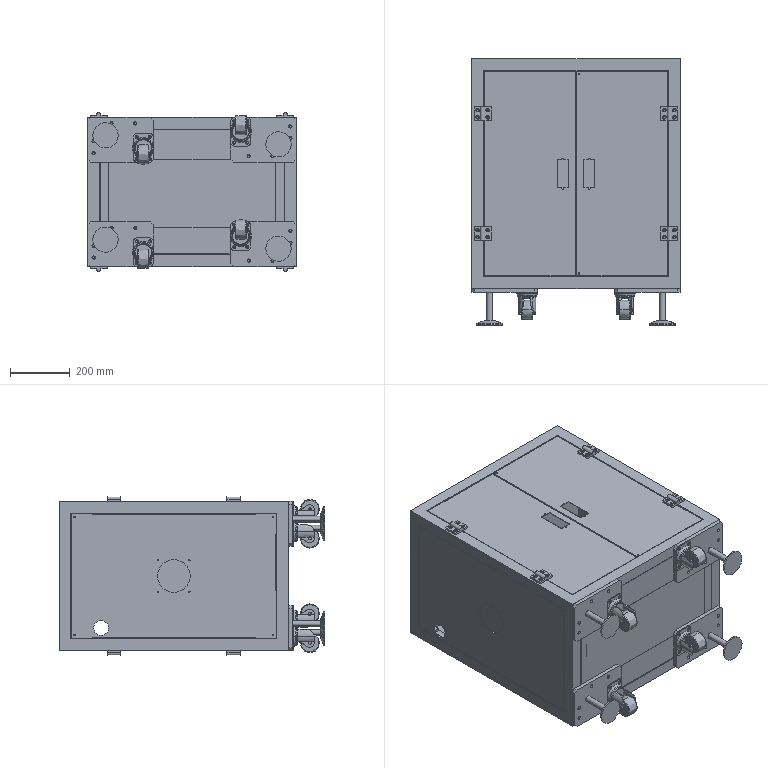Part | SolidWorks | 61 solids | 1740 faces | box 700 x 892 x 532 mm | volume 21154344 mm3 | cylinder 858 | plane 762 | cone 80 | spline 40 | commonest cylinder face diameters 1 x160 2 x96 6.6 x96 6.5 x70 4.2 x64 6.8 x32